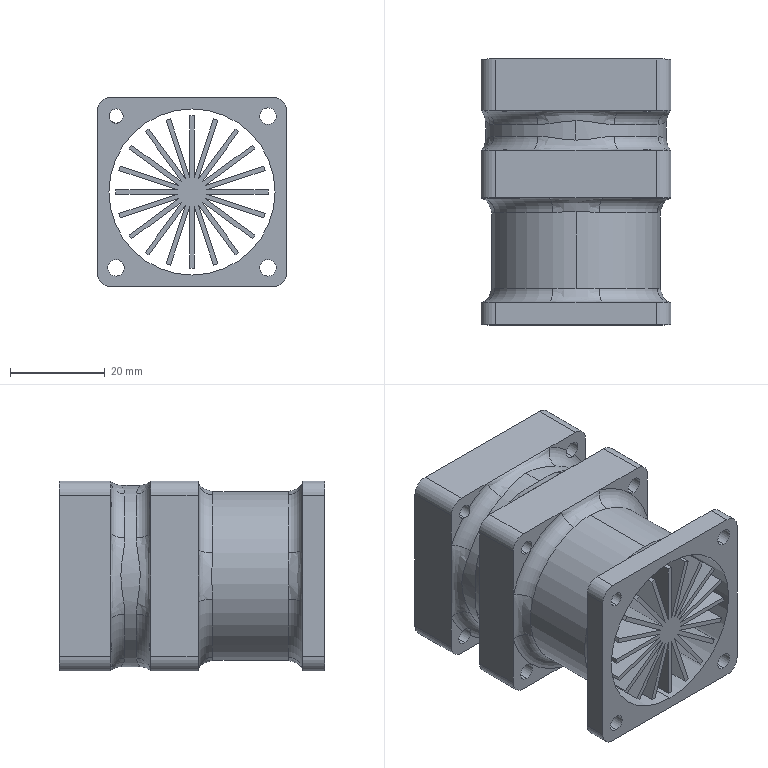Part | STEP file | Vortex fan 40 | 2 solids | 166 faces | box 40 x 56 x 40 mm | volume 33950 mm3 | plane 92 | cylinder 42 | spline 16 | torus 16 | commonest cylinder face diameters 3.5 x18 6 x12 3 x6 35 x2 35.604 x2 38.164 x2